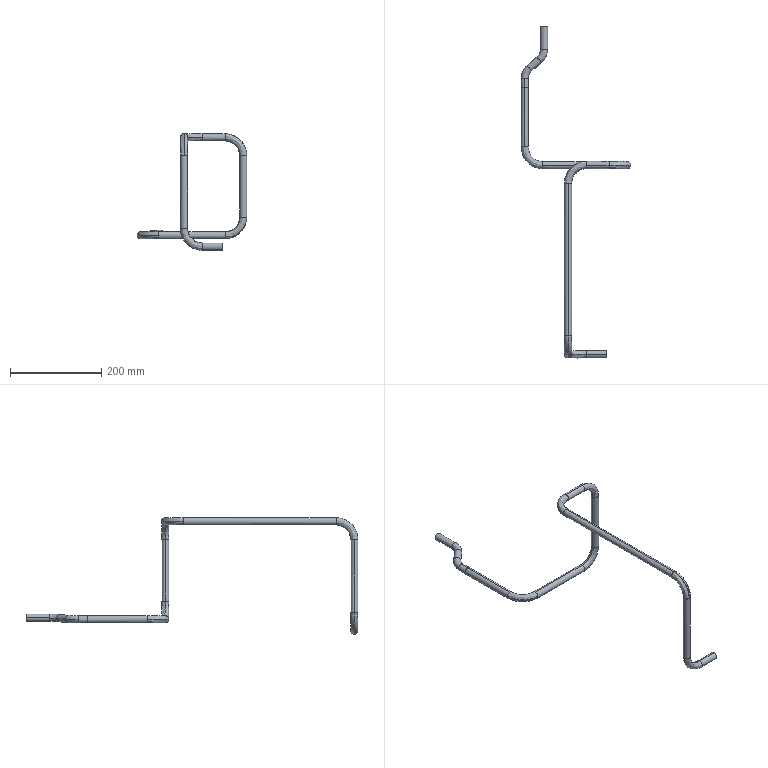Part | STEP file | copper tube 46_default_machined_ | 2 solids | 66 faces | box 241 x 728.501 x 256 mm | volume 124522 mm3 | cylinder 34 | spline 24 | plane 4 | torus 4 | commonest cylinder face diameters 16 x20 13 x14